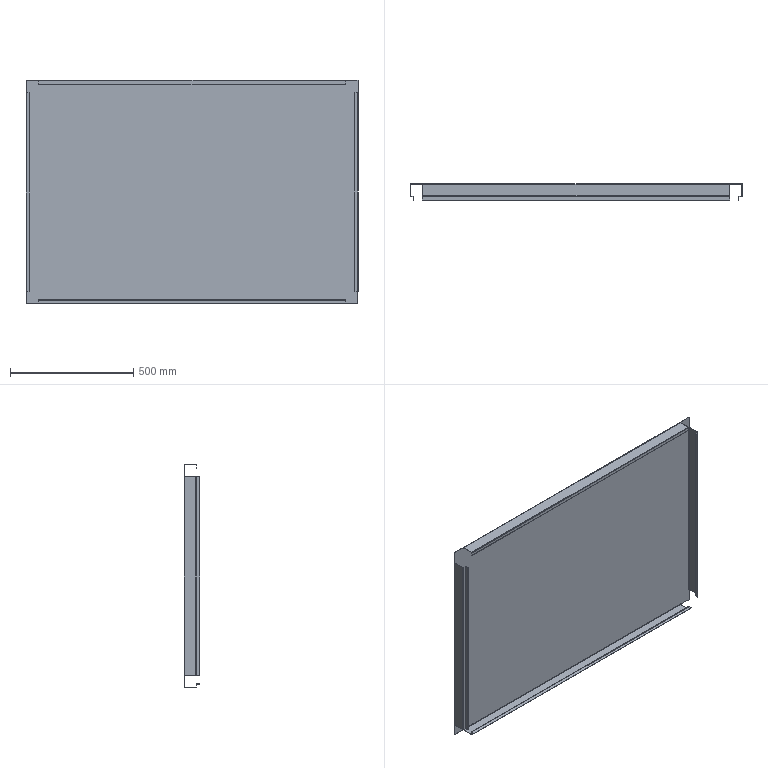Part | SolidWorks | features EdgeFlange 8, FlatPattern 1, SMBaseFlange 1, SheetMetal 1 | 1 solid | 126 faces | box 1345 x 63.8 x 904 mm | volume 1806228 mm3 | plane 104 | cylinder 22 | commonest cylinder face diameters 1.473 x11 3.873 x11